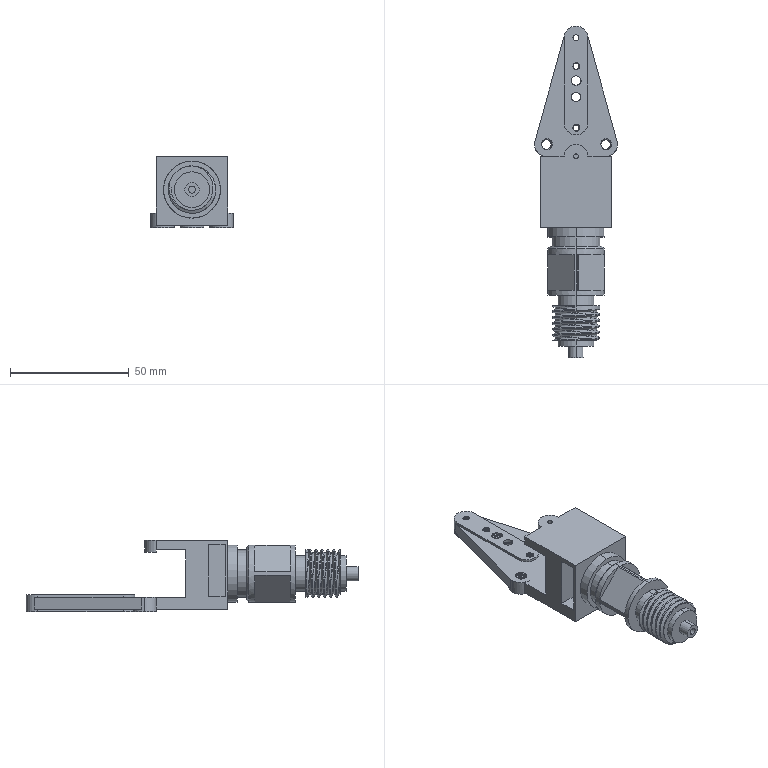Part | SolidWorks | features ICE 15, Helix 8, SweepCut 8, Cut 2, Chamfer 1, CirPattern 1, Extrusion 1 | 1 solid | 185 faces | box 35 x 140 x 30.32 mm | volume 37050 mm3 | cylinder 94 | plane 61 | spline 28 | cone 2 | commonest cylinder face diameters 4 x51 20 x15 10 x8 2.5 x6 15 x4 24 x4